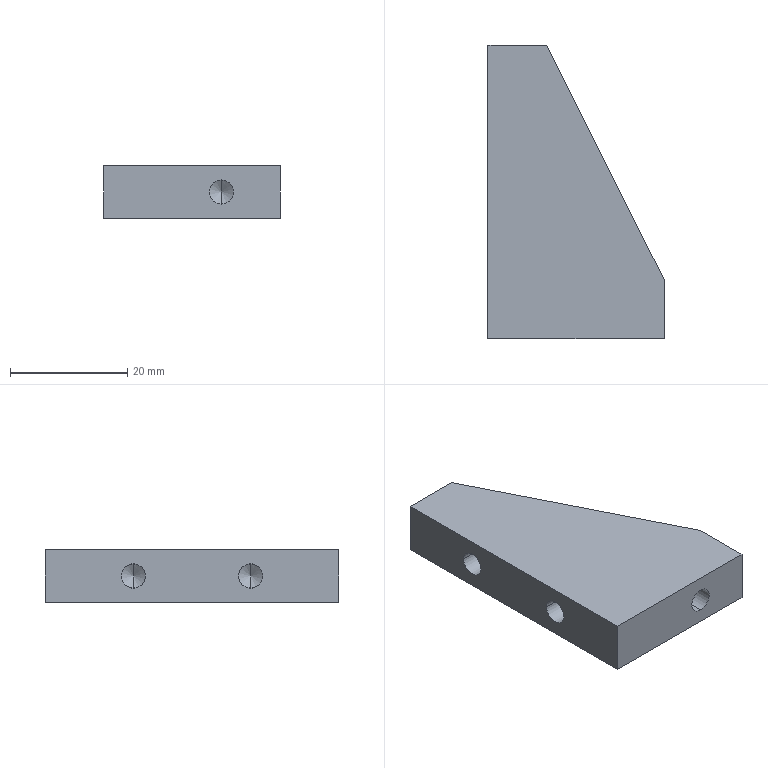Part | SolidWorks | features BaseBody 1 | 1 solid | 19 faces | box 30 x 50 x 9 mm | volume 9481 mm3 | plane 7 | cylinder 6 | cone 6 | commonest cylinder face diameters 4.134 x6
STEP:
#1=CARTESIAN_POINT('',(-31.965,-87.6,6.567));
#2=VERTEX_POINT('',#1);
#3=CARTESIAN_POINT('',(-31.965,-87.6,2.433));
#4=VERTEX_POINT('',#3);
#5=CARTESIAN_POINT('',(-31.965,-87.6,4.5));
#6=DIRECTION('',(0.,-1.,0.));
#7=DIRECTION('',(0.,0.,-1.));
#8=AXIS2_PLACEMENT_3D('',#5,#6,#7);
#9=CIRCLE('',#8,2.067);
#10=EDGE_CURVE('',#2,#4,#9,.T.);
#11=ORIENTED_EDGE('',*,*,#10,.F.);
#12=CARTESIAN_POINT('',(-31.965,-97.6,6.567));
#13=VERTEX_POINT('',#12);
#14=CARTESIAN_POINT('',(-31.965,-92.6,6.567));
#15=DIRECTION('',(0.,-1.,0.));
#16=VECTOR('',#15,1000.);
#17=LINE('',#14,#16);
#18=EDGE_CURVE('',#2,#13,#17,.T.);
#19=ORIENTED_EDGE('',*,*,#18,.T.);
#20=CARTESIAN_POINT('',(-31.965,-97.6,2.433));
#21=VERTEX_POINT('',#20);
#22=CARTESIAN_POINT('',(-31.965,-97.6,4.5));
#23=DIRECTION('',(0.,1.,0.));
#24=DIRECTION('',(0.,0.,-1.));
#25=AXIS2_PLACEMENT_3D('',#22,#23,#24);
#26=CIRCLE('',#25,2.067);
#27=EDGE_CURVE('',#21,#13,#26,.T.);
#28=ORIENTED_EDGE('',*,*,#27,.F.);
#29=CARTESIAN_POINT('',(-31.965,-92.6,2.433));
#30=DIRECTION('',(0.,-1.,0.));
#31=VECTOR('',#30,1000.);
#32=LINE('',#29,#31);
#33=EDGE_CURVE('',#4,#21,#32,.T.);
#34=ORIENTED_EDGE('',*,*,#33,.F.);
#35=EDGE_LOOP('',(#11,#19,#28,#34));
#36=FACE_OUTER_BOUND('',#35,.T.);
#37=CARTESIAN_POINT('',(-31.965,-92.6,4.5));
#38=DIRECTION('',(0.,-1.,0.));
#39=DIRECTION('',(0.,0.,-1.));
#40=AXIS2_PLACEMENT_3D('',#37,#38,#39);
#41=CYLINDRICAL_SURFACE('',#40,2.067);
#42=ADVANCED_FACE('',(#36),#41,.F.);
#43=CARTESIAN_POINT('',(-41.965,-80.533,4.5));
#44=VERTEX_POINT('',#43);
#45=CARTESIAN_POINT('',(-41.965,-82.6,2.433));
#46=VERTEX_POINT('',#45);
#47=CARTESIAN_POINT('',(-41.965,-82.6,4.5));
#48=DIRECTION('',(-1.,0.,0.));
#49=DIRECTION('',(0.,-1.,0.));
#50=AXIS2_PLACEMENT_3D('',#47,#48,#49);
#51=CIRCLE('',#50,2.067);
#52=EDGE_CURVE('',#44,#46,#51,.T.);
#53=ORIENTED_EDGE('',*,*,#52,.F.);
#54=CARTESIAN_POINT('',(-51.965,-80.533,4.5));
#55=VERTEX_POINT('',#54);
#56=CARTESIAN_POINT('',(-46.965,-80.533,4.5));
#57=DIRECTION('',(-1.,0.,0.));
#58=VECTOR('',#57,1000.);
#59=LINE('',#56,#58);
#60=EDGE_CURVE('',#44,#55,#59,.T.);
#61=ORIENTED_EDGE('',*,*,#60,.T.);
#62=CARTESIAN_POINT('',(-51.965,-84.667,4.5));
#63=VERTEX_POINT('',#62);
#64=CARTESIAN_POINT('',(-51.965,-82.6,4.5));
#65=DIRECTION('',(1.,0.,0.));
#66=DIRECTION('',(0.,-1.,0.));
#67=AXIS2_PLACEMENT_3D('',#64,#65,#66);
#68=CIRCLE('',#67,2.067);
#69=EDGE_CURVE('',#63,#55,#68,.T.);
#70=ORIENTED_EDGE('',*,*,#69,.F.);
#71=CARTESIAN_POINT('',(-41.965,-84.667,4.5));
#72=VERTEX_POINT('',#71);
#73=CARTESIAN_POINT('',(-46.965,-84.667,4.5));
#74=DIRECTION('',(-1.,0.,0.));
#75=VECTOR('',#74,1000.);
#76=LINE('',#73,#75);
#77=EDGE_CURVE('',#72,#63,#76,.T.);
#78=ORIENTED_EDGE('',*,*,#77,.F.);
#79=CARTESIAN_POINT('',(-41.965,-82.6,4.5));
#80=DIRECTION('',(-1.,0.,0.));
#81=DIRECTION('',(0.,-1.,0.));
#82=AXIS2_PLACEMENT_3D('',#79,#80,#81);
#83=CIRCLE('',#82,2.067);
#84=EDGE_CURVE('',#46,#72,#83,.T.);
#85=ORIENTED_EDGE('',*,*,#84,.F.);
#86=EDGE_LOOP('',(#53,#61,#70,#78,#85));
#87=FACE_OUTER_BOUND('',#86,.T.);
#88=CARTESIAN_POINT('',(-46.965,-82.6,4.5));
#89=DIRECTION('',(-1.,0.,0.));
#90=DIRECTION('',(0.,-1.,0.));
#91=AXIS2_PLACEMENT_3D('',#88,#89,#90);
#92=CYLINDRICAL_SURFACE('',#91,2.067);
#93=ADVANCED_FACE('',(#87),#92,.F.);
#94=CARTESIAN_POINT('',(-41.965,-60.533,4.5));
#95=VERTEX_POINT('',#94);
#96=CARTESIAN_POINT('',(-41.965,-62.6,2.433));
#97=VERTEX_POINT('',#96);
#98=CARTESIAN_POINT('',(-41.965,-62.6,4.5));
#99=DIRECTION('',(-1.,0.,0.));
#100=DIRECTION('',(0.,-1.,0.));
#101=AXIS2_PLACEMENT_3D('',#98,#99,#100);
#102=CIRCLE('',#101,2.067);
#103=EDGE_CURVE('',#95,#97,#102,.T.);
#104=ORIENTED_EDGE('',*,*,#103,.F.);
#105=CARTESIAN_POINT('',(-51.965,-60.533,4.5));
#106=VERTEX_POINT('',#105);
#107=CARTESIAN_POINT('',(-46.965,-60.533,4.5));
#108=DIRECTION('',(-1.,0.,0.));
#109=VECTOR('',#108,1000.);
#110=LINE('',#107,#109);
#111=EDGE_CURVE('',#95,#106,#110,.T.);
#112=ORIENTED_EDGE('',*,*,#111,.T.);
#113=CARTESIAN_POINT('',(-51.965,-64.667,4.5));
#114=VERTEX_POINT('',#113);
#115=CARTESIAN_POINT('',(-51.965,-62.6,4.5));
#116=DIRECTION('',(1.,0.,0.));
#117=DIRECTION('',(0.,-1.,0.));
#118=AXIS2_PLACEMENT_3D('',#115,#116,#117);
#119=CIRCLE('',#118,2.067);
#120=EDGE_CURVE('',#114,#106,#119,.T.);
#121=ORIENTED_EDGE('',*,*,#120,.F.);
#122=CARTESIAN_POINT('',(-41.965,-64.667,4.5));
#123=VERTEX_POINT('',#122);
#124=CARTESIAN_POINT('',(-46.965,-64.667,4.5));
#125=DIRECTION('',(-1.,0.,0.));
#126=VECTOR('',#125,1000.);
#127=LINE('',#124,#126);
#128=EDGE_CURVE('',#123,#114,#127,.T.);
#129=ORIENTED_EDGE('',*,*,#128,.F.);
#130=CARTESIAN_POINT('',(-41.965,-62.6,4.5));
#131=DIRECTION('',(-1.,0.,0.));
#132=DIRECTION('',(0.,-1.,0.));
#133=AXIS2_PLACEMENT_3D('',#130,#131,#132);
#134=CIRCLE('',#133,2.067);
#135=EDGE_CURVE('',#97,#123,#134,.T.);
#136=ORIENTED_EDGE('',*,*,#135,.F.);
#137=EDGE_LOOP('',(#104,#112,#121,#129,#136));
#138=FACE_OUTER_BOUND('',#137,.T.);
#139=CARTESIAN_POINT('',(-46.965,-62.6,4.5));
#140=DIRECTION('',(-1.,0.,0.));
#141=DIRECTION('',(0.,-1.,0.));
#142=AXIS2_PLACEMENT_3D('',#139,#140,#141);
#143=CYLINDRICAL_SURFACE('',#142,2.067);
#144=ADVANCED_FACE('',(#138),#143,.F.);
#145=CARTESIAN_POINT('',(-31.965,-86.358,4.5));
#146=VERTEX_POINT('',#145);
#147=CARTESIAN_POINT('',(-31.965,-87.6,2.433));
#148=DIRECTION('',(0.,-0.515,-0.8572));
#149=VECTOR('',#148,1000.);
#150=LINE('',#147,#149);
#151=EDGE_CURVE('',#146,#4,#150,.T.);
#152=ORIENTED_EDGE('',*,*,#151,.F.);
#153=CARTESIAN_POINT('',(-31.965,-87.6,6.567));
#154=DIRECTION('',(0.,-0.515,0.8572));
#155=VECTOR('',#154,1000.);
#156=LINE('',#153,#155);
#157=EDGE_CURVE('',#146,#2,#156,.T.);
#158=ORIENTED_EDGE('',*,*,#157,.T.);
#159=ORIENTED_EDGE('',*,*,#10,.T.);
#160=EDGE_LOOP('',(#152,#158,#159));
#161=FACE_OUTER_BOUND('',#160,.T.);
#162=CARTESIAN_POINT('',(-31.965,-87.6,4.5));
#163=DIRECTION('',(0.,-1.,0.));
#164=DIRECTION('',(0.,0.,-1.));
#165=AXIS2_PLACEMENT_3D('',#162,#163,#164);
#166=CONICAL_SURFACE('',#165,2.067,1.03);
#167=ADVANCED_FACE('',(#161),#166,.F.);
#168=CARTESIAN_POINT('',(-40.723,-82.6,4.5));
#169=VERTEX_POINT('',#168);
#170=CARTESIAN_POINT('',(-41.965,-82.6,6.567));
#171=VERTEX_POINT('',#170);
#172=CARTESIAN_POINT('',(-41.965,-82.6,6.567));
#173=DIRECTION('',(-0.515,0.,0.8572));
#174=VECTOR('',#173,1000.);
#175=LINE('',#172,#174);
#176=EDGE_CURVE('',#169,#171,#175,.T.);
#177=ORIENTED_EDGE('',*,*,#176,.F.);
#178=CARTESIAN_POINT('',(-41.965,-82.6,2.433));
#179=DIRECTION('',(-0.515,0.,-0.8572));
#180=VECTOR('',#179,1000.);
#181=LINE('',#178,#180);
#182=EDGE_CURVE('',#169,#46,#181,.T.);
#183=ORIENTED_EDGE('',*,*,#182,.T.);
#184=ORIENTED_EDGE('',*,*,#84,.T.);
#185=CARTESIAN_POINT('',(-41.965,-82.6,4.5));
#186=DIRECTION('',(-1.,0.,0.));
#187=DIRECTION('',(0.,-1.,0.));
#188=AXIS2_PLACEMENT_3D('',#185,#186,#187);
#189=CIRCLE('',#188,2.067);
#190=EDGE_CURVE('',#72,#171,#189,.T.);
#191=ORIENTED_EDGE('',*,*,#190,.T.);
#192=EDGE_LOOP('',(#177,#183,#184,#191));
#193=FACE_OUTER_BOUND('',#192,.T.);
#194=CARTESIAN_POINT('',(-41.965,-82.6,4.5));
#195=DIRECTION('',(-1.,0.,0.));
#196=DIRECTION('',(0.,0.,1.));
#197=AXIS2_PLACEMENT_3D('',#194,#195,#196);
#198=CONICAL_SURFACE('',#197,2.067,1.03);
#199=ADVANCED_FACE('',(#193),#198,.F.);
#200=CARTESIAN_POINT('',(-40.723,-62.6,4.5));
#201=VERTEX_POINT('',#200);
#202=CARTESIAN_POINT('',(-41.965,-62.6,6.567));
#203=VERTEX_POINT('',#202);
#204=CARTESIAN_POINT('',(-41.965,-62.6,6.567));
#205=DIRECTION('',(-0.515,0.,0.8572));
#206=VECTOR('',#205,1000.);
#207=LINE('',#204,#206);
#208=EDGE_CURVE('',#201,#203,#207,.T.);
#209=ORIENTED_EDGE('',*,*,#208,.F.);
#210=CARTESIAN_POINT('',(-41.965,-62.6,2.433));
#211=DIRECTION('',(-0.515,0.,-0.8572));
#212=VECTOR('',#211,1000.);
#213=LINE('',#210,#212);
#214=EDGE_CURVE('',#201,#97,#213,.T.);
#215=ORIENTED_EDGE('',*,*,#214,.T.);
#216=ORIENTED_EDGE('',*,*,#135,.T.);
#217=CARTESIAN_POINT('',(-41.965,-62.6,4.5));
#218=DIRECTION('',(-1.,0.,0.));
#219=DIRECTION('',(0.,-1.,0.));
#220=AXIS2_PLACEMENT_3D('',#217,#218,#219);
#221=CIRCLE('',#220,2.067);
#222=EDGE_CURVE('',#123,#203,#221,.T.);
#223=ORIENTED_EDGE('',*,*,#222,.T.);
#224=EDGE_LOOP('',(#209,#215,#216,#223));
#225=FACE_OUTER_BOUND('',#224,.T.);
#226=CARTESIAN_POINT('',(-41.965,-62.6,4.5));
#227=DIRECTION('',(-1.,0.,0.));
#228=DIRECTION('',(0.,0.,1.));
#229=AXIS2_PLACEMENT_3D('',#226,#227,#228);
#230=CONICAL_SURFACE('',#229,2.067,1.03);
#231=ADVANCED_FACE('',(#225),#230,.F.);
#232=CARTESIAN_POINT('',(-51.965,-97.6,9.));
#233=VERTEX_POINT('',#232);
#234=CARTESIAN_POINT('',(-21.965,-97.6,9.));
#235=VERTEX_POINT('',#234);
#236=CARTESIAN_POINT('',(-36.965,-97.6,9.));
#237=DIRECTION('',(1.,0.,0.));
#238=VECTOR('',#237,1000.);
#239=LINE('',#236,#238);
#240=EDGE_CURVE('',#233,#235,#239,.T.);
#241=ORIENTED_EDGE('',*,*,#240,.T.);
#242=CARTESIAN_POINT('',(-21.965,-87.6,9.));
#243=VERTEX_POINT('',#242);
#244=CARTESIAN_POINT('',(-21.965,-72.6,9.));
#245=DIRECTION('',(0.,1.,0.));
#246=VECTOR('',#245,1000.);
#247=LINE('',#244,#246);
#248=EDGE_CURVE('',#235,#243,#247,.T.);
#249=ORIENTED_EDGE('',*,*,#248,.T.);
#250=CARTESIAN_POINT('',(-41.965,-47.6,9.));
#251=VERTEX_POINT('',#250);
#252=CARTESIAN_POINT('',(-21.965,-87.6,9.));
#253=DIRECTION('',(-0.4472,0.8944,0.));
#254=VECTOR('',#253,1000.);
#255=LINE('',#252,#254);
#256=EDGE_CURVE('',#243,#251,#255,.T.);
#257=ORIENTED_EDGE('',*,*,#256,.T.);
#258=CARTESIAN_POINT('',(-51.965,-47.6,9.));
#259=VERTEX_POINT('',#258);
#260=CARTESIAN_POINT('',(-36.965,-47.6,9.));
#261=DIRECTION('',(-1.,0.,0.));
#262=VECTOR('',#261,1000.);
#263=LINE('',#260,#262);
#264=EDGE_CURVE('',#251,#259,#263,.T.);
#265=ORIENTED_EDGE('',*,*,#264,.T.);
#266=CARTESIAN_POINT('',(-51.965,-72.6,9.));
#267=DIRECTION('',(0.,-1.,0.));
#268=VECTOR('',#267,1000.);
#269=LINE('',#266,#268);
#270=EDGE_CURVE('',#259,#233,#269,.T.);
#271=ORIENTED_EDGE('',*,*,#270,.T.);
#272=EDGE_LOOP('',(#241,#249,#257,#265,#271));
#273=FACE_OUTER_BOUND('',#272,.T.);
#274=CARTESIAN_POINT('',(-36.965,-72.6,9.));
#275=DIRECTION('',(0.,0.,1.));
#276=DIRECTION('',(1.,0.,0.));
#277=AXIS2_PLACEMENT_3D('',#274,#275,#276);
#278=PLANE('',#277);
#279=ADVANCED_FACE('',(#273),#278,.T.);
#280=CARTESIAN_POINT('',(-21.965,-97.6,0.));
#281=VERTEX_POINT('',#280);
#282=CARTESIAN_POINT('',(-21.965,-97.6,0.));
#283=DIRECTION('',(0.,0.,-1.));
#284=VECTOR('',#283,1000.);
#285=LINE('',#282,#284);
#286=EDGE_CURVE('',#235,#281,#285,.T.);
#287=ORIENTED_EDGE('',*,*,#286,.T.);
#288=CARTESIAN_POINT('',(-21.965,-87.6,0.));
#289=VERTEX_POINT('',#288);
#290=CARTESIAN_POINT('',(-21.965,-47.6,0.));
#291=DIRECTION('',(0.,1.,0.));
#292=VECTOR('',#291,1000.);
#293=LINE('',#290,#292);
#294=EDGE_CURVE('',#281,#289,#293,.T.);
#295=ORIENTED_EDGE('',*,*,#294,.T.);
#296=CARTESIAN_POINT('',(-21.965,-87.6,0.));
#297=DIRECTION('',(0.,0.,1.));
#298=VECTOR('',#297,1000.);
#299=LINE('',#296,#298);
#300=EDGE_CURVE('',#289,#243,#299,.T.);
#301=ORIENTED_EDGE('',*,*,#300,.T.);
#302=ORIENTED_EDGE('',*,*,#248,.F.);
#303=EDGE_LOOP('',(#287,#295,#301,#302));
#304=FACE_OUTER_BOUND('',#303,.T.);
#305=CARTESIAN_POINT('',(-21.965,-47.6,0.));
#306=DIRECTION('',(1.,0.,0.));
#307=DIRECTION('',(0.,0.,-1.));
#308=AXIS2_PLACEMENT_3D('',#305,#306,#307);
#309=PLANE('',#308);
#310=ADVANCED_FACE('',(#304),#309,.T.);
#311=ORIENTED_EDGE('',*,*,#27,.T.);
#312=CARTESIAN_POINT('',(-31.965,-97.6,4.5));
#313=DIRECTION('',(0.,1.,0.));
#314=DIRECTION('',(0.,0.,-1.));
#315=AXIS2_PLACEMENT_3D('',#312,#313,#314);
#316=CIRCLE('',#315,2.067);
#317=EDGE_CURVE('',#13,#21,#316,.T.);
#318=ORIENTED_EDGE('',*,*,#317,.T.);
#319=EDGE_LOOP('',(#311,#318));
#320=FACE_BOUND('',#319,.T.);
#321=CARTESIAN_POINT('',(-51.965,-97.6,0.));
#322=VERTEX_POINT('',#321);
#323=CARTESIAN_POINT('',(-21.965,-97.6,0.));
#324=DIRECTION('',(1.,0.,0.));
#325=VECTOR('',#324,1000.);
#326=LINE('',#323,#325);
#327=EDGE_CURVE('',#322,#281,#326,.T.);
#328=ORIENTED_EDGE('',*,*,#327,.T.);
#329=ORIENTED_EDGE('',*,*,#286,.F.);
#330=ORIENTED_EDGE('',*,*,#240,.F.);
#331=CARTESIAN_POINT('',(-51.965,-97.6,0.));
#332=DIRECTION('',(0.,0.,-1.));
#333=VECTOR('',#332,1000.);
#334=LINE('',#331,#333);
#335=EDGE_CURVE('',#233,#322,#334,.T.);
#336=ORIENTED_EDGE('',*,*,#335,.T.);
#337=EDGE_LOOP('',(#328,#329,#330,#336));
#338=FACE_OUTER_BOUND('',#337,.T.);
#339=CARTESIAN_POINT('',(-21.965,-97.6,0.));
#340=DIRECTION('',(0.,-1.,0.));
#341=DIRECTION('',(0.,0.,-1.));
#342=AXIS2_PLACEMENT_3D('',#339,#340,#341);
#343=PLANE('',#342);
#344=ADVANCED_FACE('',(#320,#338),#343,.T.);
#345=ORIENTED_EDGE('',*,*,#69,.T.);
#346=CARTESIAN_POINT('',(-51.965,-82.6,4.5));
#347=DIRECTION('',(1.,0.,0.));
#348=DIRECTION('',(0.,-1.,0.));
#349=AXIS2_PLACEMENT_3D('',#346,#347,#348);
#350=CIRCLE('',#349,2.067);
#351=EDGE_CURVE('',#55,#63,#350,.T.);
#352=ORIENTED_EDGE('',*,*,#351,.T.);
#353=EDGE_LOOP('',(#345,#352));
#354=FACE_BOUND('',#353,.T.);
#355=ORIENTED_EDGE('',*,*,#120,.T.);
#356=CARTESIAN_POINT('',(-51.965,-62.6,4.5));
#357=DIRECTION('',(1.,0.,0.));
#358=DIRECTION('',(0.,-1.,0.));
#359=AXIS2_PLACEMENT_3D('',#356,#357,#358);
#360=CIRCLE('',#359,2.067);
#361=EDGE_CURVE('',#106,#114,#360,.T.);
#362=ORIENTED_EDGE('',*,*,#361,.T.);
#363=EDGE_LOOP('',(#355,#362));
#364=FACE_BOUND('',#363,.T.);
#365=CARTESIAN_POINT('',(-51.965,-47.6,0.));
#366=VERTEX_POINT('',#365);
#367=CARTESIAN_POINT('',(-51.965,-97.6,0.));
#368=DIRECTION('',(0.,-1.,0.));
#369=VECTOR('',#368,1000.);
#370=LINE('',#367,#369);
#371=EDGE_CURVE('',#366,#322,#370,.T.);
#372=ORIENTED_EDGE('',*,*,#371,.T.);
#373=ORIENTED_EDGE('',*,*,#335,.F.);
#374=ORIENTED_EDGE('',*,*,#270,.F.);
#375=CARTESIAN_POINT('',(-51.965,-47.6,0.));
#376=DIRECTION('',(0.,0.,-1.));
#377=VECTOR('',#376,1000.);
#378=LINE('',#375,#377);
#379=EDGE_CURVE('',#259,#366,#378,.T.);
#380=ORIENTED_EDGE('',*,*,#379,.T.);
#381=EDGE_LOOP('',(#372,#373,#374,#380));
#382=FACE_OUTER_BOUND('',#381,.T.);
#383=CARTESIAN_POINT('',(-51.965,-97.6,0.));
#384=DIRECTION('',(-1.,0.,0.));
#385=DIRECTION('',(0.,0.,1.));
#386=AXIS2_PLACEMENT_3D('',#383,#384,#385);
#387=PLANE('',#386);
#388=ADVANCED_FACE('',(#354,#364,#382),#387,.T.);
#389=ORIENTED_EDGE('',*,*,#379,.F.);
#390=ORIENTED_EDGE('',*,*,#264,.F.);
#391=CARTESIAN_POINT('',(-41.965,-47.6,0.));
#392=VERTEX_POINT('',#391);
#393=CARTESIAN_POINT('',(-41.965,-47.6,0.));
#394=DIRECTION('',(0.,0.,-1.));
#395=VECTOR('',#394,1000.);
#396=LINE('',#393,#395);
#397=EDGE_CURVE('',#251,#392,#396,.T.);
#398=ORIENTED_EDGE('',*,*,#397,.T.);
#399=CARTESIAN_POINT('',(-51.965,-47.6,0.));
#400=DIRECTION('',(-1.,0.,0.));
#401=VECTOR('',#400,1000.);
#402=LINE('',#399,#401);
#403=EDGE_CURVE('',#392,#366,#402,.T.);
#404=ORIENTED_EDGE('',*,*,#403,.T.);
#405=EDGE_LOOP('',(#389,#390,#398,#404));
#406=FACE_OUTER_BOUND('',#405,.T.);
#407=CARTESIAN_POINT('',(-51.965,-47.6,0.));
#408=DIRECTION('',(0.,1.,0.));
#409=DIRECTION('',(0.,0.,1.));
#410=AXIS2_PLACEMENT_3D('',#407,#408,#409);
#411=PLANE('',#410);
#412=ADVANCED_FACE('',(#406),#411,.T.);
#413=CARTESIAN_POINT('',(-31.965,-67.6,0.));
#414=DIRECTION('',(-0.4472,0.8944,0.));
#415=VECTOR('',#414,1000.);
#416=LINE('',#413,#415);
#417=EDGE_CURVE('',#289,#392,#416,.T.);
#418=ORIENTED_EDGE('',*,*,#417,.T.);
#419=ORIENTED_EDGE('',*,*,#397,.F.);
#420=ORIENTED_EDGE('',*,*,#256,.F.);
#421=ORIENTED_EDGE('',*,*,#300,.F.);
#422=EDGE_LOOP('',(#418,#419,#420,#421));
#423=FACE_OUTER_BOUND('',#422,.T.);
#424=CARTESIAN_POINT('',(-31.965,-67.6,0.));
#425=DIRECTION('',(0.8944,0.4472,0.));
#426=DIRECTION('',(-0.4472,0.8944,0.));
#427=AXIS2_PLACEMENT_3D('',#424,#425,#426);
#428=PLANE('',#427);
#429=ADVANCED_FACE('',(#423),#428,.T.);
#430=ORIENTED_EDGE('',*,*,#294,.F.);
#431=ORIENTED_EDGE('',*,*,#327,.F.);
#432=ORIENTED_EDGE('',*,*,#371,.F.);
#433=ORIENTED_EDGE('',*,*,#403,.F.);
#434=ORIENTED_EDGE('',*,*,#417,.F.);
#435=EDGE_LOOP('',(#430,#431,#432,#433,#434));
#436=FACE_OUTER_BOUND('',#435,.T.);
#437=CARTESIAN_POINT('',(-36.965,-72.6,0.));
#438=DIRECTION('',(0.,0.,1.));
#439=DIRECTION('',(1.,0.,0.));
#440=AXIS2_PLACEMENT_3D('',#437,#438,#439);
#441=PLANE('',#440);
#442=ADVANCED_FACE('',(#436),#441,.F.);
#443=ORIENTED_EDGE('',*,*,#18,.F.);
#444=CARTESIAN_POINT('',(-31.965,-87.6,4.5));
#445=DIRECTION('',(0.,-1.,0.));
#446=DIRECTION('',(0.,0.,-1.));
#447=AXIS2_PLACEMENT_3D('',#444,#445,#446);
#448=CIRCLE('',#447,2.067);
#449=EDGE_CURVE('',#4,#2,#448,.T.);
#450=ORIENTED_EDGE('',*,*,#449,.F.);
#451=ORIENTED_EDGE('',*,*,#33,.T.);
#452=ORIENTED_EDGE('',*,*,#317,.F.);
#453=EDGE_LOOP('',(#443,#450,#451,#452));
#454=FACE_OUTER_BOUND('',#453,.T.);
#455=CARTESIAN_POINT('',(-31.965,-92.6,4.5));
#456=DIRECTION('',(0.,-1.,0.));
#457=DIRECTION('',(0.,0.,-1.));
#458=AXIS2_PLACEMENT_3D('',#455,#456,#457);
#459=CYLINDRICAL_SURFACE('',#458,2.067);
#460=ADVANCED_FACE('',(#454),#459,.F.);
#461=ORIENTED_EDGE('',*,*,#60,.F.);
#462=CARTESIAN_POINT('',(-41.965,-82.6,4.5));
#463=DIRECTION('',(-1.,0.,0.));
#464=DIRECTION('',(0.,-1.,0.));
#465=AXIS2_PLACEMENT_3D('',#462,#463,#464);
#466=CIRCLE('',#465,2.067);
#467=EDGE_CURVE('',#171,#44,#466,.T.);
#468=ORIENTED_EDGE('',*,*,#467,.F.);
#469=ORIENTED_EDGE('',*,*,#190,.F.);
#470=ORIENTED_EDGE('',*,*,#77,.T.);
#471=ORIENTED_EDGE('',*,*,#351,.F.);
#472=EDGE_LOOP('',(#461,#468,#469,#470,#471));
#473=FACE_OUTER_BOUND('',#472,.T.);
#474=CARTESIAN_POINT('',(-46.965,-82.6,4.5));
#475=DIRECTION('',(-1.,0.,0.));
#476=DIRECTION('',(0.,-1.,0.));
#477=AXIS2_PLACEMENT_3D('',#474,#475,#476);
#478=CYLINDRICAL_SURFACE('',#477,2.067);
#479=ADVANCED_FACE('',(#473),#478,.F.);
#480=ORIENTED_EDGE('',*,*,#111,.F.);
#481=CARTESIAN_POINT('',(-41.965,-62.6,4.5));
#482=DIRECTION('',(-1.,0.,0.));
#483=DIRECTION('',(0.,-1.,0.));
#484=AXIS2_PLACEMENT_3D('',#481,#482,#483);
#485=CIRCLE('',#484,2.067);
#486=EDGE_CURVE('',#203,#95,#485,.T.);
#487=ORIENTED_EDGE('',*,*,#486,.F.);
#488=ORIENTED_EDGE('',*,*,#222,.F.);
#489=ORIENTED_EDGE('',*,*,#128,.T.);
#490=ORIENTED_EDGE('',*,*,#361,.F.);
#491=EDGE_LOOP('',(#480,#487,#488,#489,#490));
#492=FACE_OUTER_BOUND('',#491,.T.);
#493=CARTESIAN_POINT('',(-46.965,-62.6,4.5));
#494=DIRECTION('',(-1.,0.,0.));
#495=DIRECTION('',(0.,-1.,0.));
#496=AXIS2_PLACEMENT_3D('',#493,#494,#495);
#497=CYLINDRICAL_SURFACE('',#496,2.067);
#498=ADVANCED_FACE('',(#492),#497,.F.);
#499=ORIENTED_EDGE('',*,*,#157,.F.);
#500=ORIENTED_EDGE('',*,*,#151,.T.);
#501=ORIENTED_EDGE('',*,*,#449,.T.);
#502=EDGE_LOOP('',(#499,#500,#501));
#503=FACE_OUTER_BOUND('',#502,.T.);
#504=CARTESIAN_POINT('',(-31.965,-87.6,4.5));
#505=DIRECTION('',(0.,-1.,0.));
#506=DIRECTION('',(0.,0.,-1.));
#507=AXIS2_PLACEMENT_3D('',#504,#505,#506);
#508=CONICAL_SURFACE('',#507,2.067,1.03);
#509=ADVANCED_FACE('',(#503),#508,.F.);
#510=ORIENTED_EDGE('',*,*,#182,.F.);
#511=ORIENTED_EDGE('',*,*,#176,.T.);
#512=ORIENTED_EDGE('',*,*,#467,.T.);
#513=ORIENTED_EDGE('',*,*,#52,.T.);
#514=EDGE_LOOP('',(#510,#511,#512,#513));
#515=FACE_OUTER_BOUND('',#514,.T.);
#516=CARTESIAN_POINT('',(-41.965,-82.6,4.5));
#517=DIRECTION('',(-1.,0.,0.));
#518=DIRECTION('',(0.,0.,1.));
#519=AXIS2_PLACEMENT_3D('',#516,#517,#518);
#520=CONICAL_SURFACE('',#519,2.067,1.03);
#521=ADVANCED_FACE('',(#515),#520,.F.);
#522=ORIENTED_EDGE('',*,*,#214,.F.);
#523=ORIENTED_EDGE('',*,*,#208,.T.);
#524=ORIENTED_EDGE('',*,*,#486,.T.);
#525=ORIENTED_EDGE('',*,*,#103,.T.);
#526=EDGE_LOOP('',(#522,#523,#524,#525));
#527=FACE_OUTER_BOUND('',#526,.T.);
#528=CARTESIAN_POINT('',(-41.965,-62.6,4.5));
#529=DIRECTION('',(-1.,0.,0.));
#530=DIRECTION('',(0.,0.,1.));
#531=AXIS2_PLACEMENT_3D('',#528,#529,#530);
#532=CONICAL_SURFACE('',#531,2.067,1.03);
#533=ADVANCED_FACE('',(#527),#532,.F.);
#534=CLOSED_SHELL('',(#42,#93,#144,#167,#199,#231,#279,#310,#344,#388,#412,#429,#442,#460,#479,#498,#509,#521,#533));
#535=MANIFOLD_SOLID_BREP('',#534);
#536=CARTESIAN_POINT('',(0.,0.,0.));
#537=DIRECTION('',(0.,0.,1.));
#538=DIRECTION('',(1.,0.,0.));
#539=AXIS2_PLACEMENT_3D('',#536,#537,#538);
#540=(LENGTH_UNIT()NAMED_UNIT(*)SI_UNIT(.MILLI.,.METRE.));
#541=UNCERTAINTY_MEASURE_WITH_UNIT(LENGTH_MEASURE(0.00001),#540,'','');
#542=(NAMED_UNIT(*)PLANE_ANGLE_UNIT()SI_UNIT($,.RADIAN.));
#543=(NAMED_UNIT(*)SI_UNIT($,.STERADIAN.)SOLID_ANGLE_UNIT());
#544=(GEOMETRIC_REPRESENTATION_CONTEXT(3)GLOBAL_UNCERTAINTY_ASSIGNED_CONTEXT((#541))GLOBAL_UNIT_ASSIGNED_CONTEXT((#540,#542,#543))REPRESENTATION_CONTEXT('',''));
#545=ADVANCED_BREP_SHAPE_REPRESENTATION('',(#535,#539),#544);